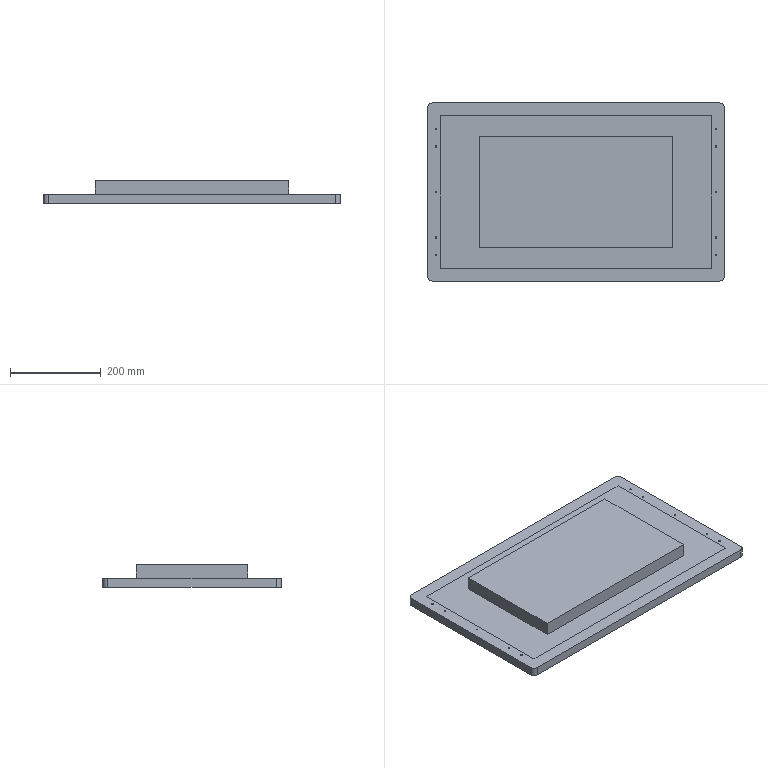Part | SolidWorks | features BaseBody 2 | 2 solids | 55 faces | box 654.7 x 392.6 x 50 mm | volume 8081843 mm3 | plane 31 | cylinder 24 | commonest cylinder face diameters 3.2 x20 20 x4
STEP:
#1=CARTESIAN_POINT('',(299.,168.,1.));
#2=VERTEX_POINT('',#1);
#3=CARTESIAN_POINT('',(299.,-168.,1.));
#4=VERTEX_POINT('',#3);
#5=CARTESIAN_POINT('',(299.,-168.,1.));
#6=DIRECTION('',(0.,-1.,0.));
#7=VECTOR('',#6,1000.);
#8=LINE('',#5,#7);
#9=EDGE_CURVE('',#2,#4,#8,.T.);
#10=ORIENTED_EDGE('',*,*,#9,.F.);
#11=CARTESIAN_POINT('',(299.,168.,20.));
#12=VERTEX_POINT('',#11);
#13=CARTESIAN_POINT('',(299.,168.,50.01));
#14=DIRECTION('',(0.,0.,-1.));
#15=VECTOR('',#14,1000.);
#16=LINE('',#13,#15);
#17=EDGE_CURVE('',#12,#2,#16,.T.);
#18=ORIENTED_EDGE('',*,*,#17,.F.);
#19=CARTESIAN_POINT('',(299.,-168.,20.));
#20=VERTEX_POINT('',#19);
#21=CARTESIAN_POINT('',(299.,0.,20.));
#22=DIRECTION('',(0.,-1.,0.));
#23=VECTOR('',#22,1000.);
#24=LINE('',#21,#23);
#25=EDGE_CURVE('',#12,#20,#24,.T.);
#26=ORIENTED_EDGE('',*,*,#25,.T.);
#27=CARTESIAN_POINT('',(299.,-168.,50.01));
#28=DIRECTION('',(0.,0.,-1.));
#29=VECTOR('',#28,1000.);
#30=LINE('',#27,#29);
#31=EDGE_CURVE('',#20,#4,#30,.T.);
#32=ORIENTED_EDGE('',*,*,#31,.T.);
#33=EDGE_LOOP('',(#10,#18,#26,#32));
#34=FACE_OUTER_BOUND('',#33,.T.);
#35=CARTESIAN_POINT('',(299.,168.,50.01));
#36=DIRECTION('',(1.,0.,0.));
#37=DIRECTION('',(0.,1.,0.));
#38=AXIS2_PLACEMENT_3D('',#35,#36,#37);
#39=PLANE('',#38);
#40=ADVANCED_FACE('',(#34),#39,.T.);
#41=CARTESIAN_POINT('',(-299.,168.,1.));
#42=VERTEX_POINT('',#41);
#43=CARTESIAN_POINT('',(299.,168.,1.));
#44=DIRECTION('',(1.,0.,0.));
#45=VECTOR('',#44,1000.);
#46=LINE('',#43,#45);
#47=EDGE_CURVE('',#42,#2,#46,.T.);
#48=ORIENTED_EDGE('',*,*,#47,.F.);
#49=CARTESIAN_POINT('',(-299.,168.,20.));
#50=VERTEX_POINT('',#49);
#51=CARTESIAN_POINT('',(-299.,168.,50.01));
#52=DIRECTION('',(0.,0.,-1.));
#53=VECTOR('',#52,1000.);
#54=LINE('',#51,#53);
#55=EDGE_CURVE('',#50,#42,#54,.T.);
#56=ORIENTED_EDGE('',*,*,#55,.F.);
#57=CARTESIAN_POINT('',(0.,168.,20.));
#58=DIRECTION('',(1.,0.,0.));
#59=VECTOR('',#58,1000.);
#60=LINE('',#57,#59);
#61=EDGE_CURVE('',#50,#12,#60,.T.);
#62=ORIENTED_EDGE('',*,*,#61,.T.);
#63=ORIENTED_EDGE('',*,*,#17,.T.);
#64=EDGE_LOOP('',(#48,#56,#62,#63));
#65=FACE_OUTER_BOUND('',#64,.T.);
#66=CARTESIAN_POINT('',(-299.,168.,50.01));
#67=DIRECTION('',(0.,1.,0.));
#68=DIRECTION('',(1.,0.,0.));
#69=AXIS2_PLACEMENT_3D('',#66,#67,#68);
#70=PLANE('',#69);
#71=ADVANCED_FACE('',(#65),#70,.T.);
#72=CARTESIAN_POINT('',(-299.,-168.,1.));
#73=VERTEX_POINT('',#72);
#74=CARTESIAN_POINT('',(-299.,-168.,1.));
#75=DIRECTION('',(0.,1.,0.));
#76=VECTOR('',#75,1000.);
#77=LINE('',#74,#76);
#78=EDGE_CURVE('',#73,#42,#77,.T.);
#79=ORIENTED_EDGE('',*,*,#78,.F.);
#80=CARTESIAN_POINT('',(-299.,-168.,20.));
#81=VERTEX_POINT('',#80);
#82=CARTESIAN_POINT('',(-299.,-168.,50.01));
#83=DIRECTION('',(0.,0.,-1.));
#84=VECTOR('',#83,1000.);
#85=LINE('',#82,#84);
#86=EDGE_CURVE('',#81,#73,#85,.T.);
#87=ORIENTED_EDGE('',*,*,#86,.F.);
#88=CARTESIAN_POINT('',(-299.,0.,20.));
#89=DIRECTION('',(0.,1.,0.));
#90=VECTOR('',#89,1000.);
#91=LINE('',#88,#90);
#92=EDGE_CURVE('',#81,#50,#91,.T.);
#93=ORIENTED_EDGE('',*,*,#92,.T.);
#94=ORIENTED_EDGE('',*,*,#55,.T.);
#95=EDGE_LOOP('',(#79,#87,#93,#94));
#96=FACE_OUTER_BOUND('',#95,.T.);
#97=CARTESIAN_POINT('',(-299.,-168.,50.01));
#98=DIRECTION('',(-1.,0.,0.));
#99=DIRECTION('',(0.,0.,1.));
#100=AXIS2_PLACEMENT_3D('',#97,#98,#99);
#101=PLANE('',#100);
#102=ADVANCED_FACE('',(#96),#101,.T.);
#103=CARTESIAN_POINT('',(299.,-168.,1.));
#104=DIRECTION('',(-1.,0.,0.));
#105=VECTOR('',#104,1000.);
#106=LINE('',#103,#105);
#107=EDGE_CURVE('',#4,#73,#106,.T.);
#108=ORIENTED_EDGE('',*,*,#107,.F.);
#109=ORIENTED_EDGE('',*,*,#31,.F.);
#110=CARTESIAN_POINT('',(0.,-168.,20.));
#111=DIRECTION('',(-1.,0.,0.));
#112=VECTOR('',#111,1000.);
#113=LINE('',#110,#112);
#114=EDGE_CURVE('',#20,#81,#113,.T.);
#115=ORIENTED_EDGE('',*,*,#114,.T.);
#116=ORIENTED_EDGE('',*,*,#86,.T.);
#117=EDGE_LOOP('',(#108,#109,#115,#116));
#118=FACE_OUTER_BOUND('',#117,.T.);
#119=CARTESIAN_POINT('',(299.,-168.,50.01));
#120=DIRECTION('',(0.,-1.,0.));
#121=DIRECTION('',(0.,0.,-1.));
#122=AXIS2_PLACEMENT_3D('',#119,#120,#121);
#123=PLANE('',#122);
#124=ADVANCED_FACE('',(#118),#123,.T.);
#125=ORIENTED_EDGE('',*,*,#78,.T.);
#126=ORIENTED_EDGE('',*,*,#47,.T.);
#127=ORIENTED_EDGE('',*,*,#9,.T.);
#128=ORIENTED_EDGE('',*,*,#107,.T.);
#129=EDGE_LOOP('',(#125,#126,#127,#128));
#130=FACE_OUTER_BOUND('',#129,.T.);
#131=CARTESIAN_POINT('',(0.,0.,1.));
#132=DIRECTION('',(0.,0.,1.));
#133=DIRECTION('',(1.,0.,0.));
#134=AXIS2_PLACEMENT_3D('',#131,#132,#133);
#135=PLANE('',#134);
#136=ADVANCED_FACE('',(#130),#135,.F.);
#137=CARTESIAN_POINT('',(213.,-123.,20.));
#138=VERTEX_POINT('',#137);
#139=CARTESIAN_POINT('',(213.,123.,20.));
#140=VERTEX_POINT('',#139);
#141=CARTESIAN_POINT('',(213.,-123.,20.));
#142=DIRECTION('',(0.,1.,0.));
#143=VECTOR('',#142,1000.);
#144=LINE('',#141,#143);
#145=EDGE_CURVE('',#138,#140,#144,.T.);
#146=ORIENTED_EDGE('',*,*,#145,.F.);
#147=CARTESIAN_POINT('',(-213.,-123.,20.));
#148=VERTEX_POINT('',#147);
#149=CARTESIAN_POINT('',(-213.,-123.,20.));
#150=DIRECTION('',(1.,0.,0.));
#151=VECTOR('',#150,1000.);
#152=LINE('',#149,#151);
#153=EDGE_CURVE('',#148,#138,#152,.T.);
#154=ORIENTED_EDGE('',*,*,#153,.F.);
#155=CARTESIAN_POINT('',(-213.,123.,20.));
#156=VERTEX_POINT('',#155);
#157=CARTESIAN_POINT('',(-213.,-123.,20.));
#158=DIRECTION('',(0.,-1.,0.));
#159=VECTOR('',#158,1000.);
#160=LINE('',#157,#159);
#161=EDGE_CURVE('',#156,#148,#160,.T.);
#162=ORIENTED_EDGE('',*,*,#161,.F.);
#163=CARTESIAN_POINT('',(-213.,123.,20.));
#164=DIRECTION('',(-1.,0.,0.));
#165=VECTOR('',#164,1000.);
#166=LINE('',#163,#165);
#167=EDGE_CURVE('',#140,#156,#166,.T.);
#168=ORIENTED_EDGE('',*,*,#167,.F.);
#169=EDGE_LOOP('',(#146,#154,#162,#168));
#170=FACE_BOUND('',#169,.T.);
#171=ORIENTED_EDGE('',*,*,#114,.F.);
#172=ORIENTED_EDGE('',*,*,#25,.F.);
#173=ORIENTED_EDGE('',*,*,#61,.F.);
#174=ORIENTED_EDGE('',*,*,#92,.F.);
#175=EDGE_LOOP('',(#171,#172,#173,#174));
#176=FACE_OUTER_BOUND('',#175,.T.);
#177=CARTESIAN_POINT('',(0.,0.,20.));
#178=DIRECTION('',(0.,0.,-1.));
#179=DIRECTION('',(0.,-1.,0.));
#180=AXIS2_PLACEMENT_3D('',#177,#178,#179);
#181=PLANE('',#180);
#182=ADVANCED_FACE('',(#170,#176),#181,.F.);
#183=ORIENTED_EDGE('',*,*,#145,.T.);
#184=CARTESIAN_POINT('',(213.,123.,50.));
#185=VERTEX_POINT('',#184);
#186=CARTESIAN_POINT('',(213.,123.,50.));
#187=DIRECTION('',(0.,0.,-1.));
#188=VECTOR('',#187,1000.);
#189=LINE('',#186,#188);
#190=EDGE_CURVE('',#185,#140,#189,.T.);
#191=ORIENTED_EDGE('',*,*,#190,.F.);
#192=CARTESIAN_POINT('',(213.,-123.,50.));
#193=VERTEX_POINT('',#192);
#194=CARTESIAN_POINT('',(213.,-123.,50.));
#195=DIRECTION('',(0.,1.,0.));
#196=VECTOR('',#195,1000.);
#197=LINE('',#194,#196);
#198=EDGE_CURVE('',#193,#185,#197,.T.);
#199=ORIENTED_EDGE('',*,*,#198,.F.);
#200=CARTESIAN_POINT('',(213.,-123.,50.));
#201=DIRECTION('',(0.,0.,-1.));
#202=VECTOR('',#201,1000.);
#203=LINE('',#200,#202);
#204=EDGE_CURVE('',#193,#138,#203,.T.);
#205=ORIENTED_EDGE('',*,*,#204,.T.);
#206=EDGE_LOOP('',(#183,#191,#199,#205));
#207=FACE_OUTER_BOUND('',#206,.T.);
#208=CARTESIAN_POINT('',(213.,-123.,50.));
#209=DIRECTION('',(-1.,0.,0.));
#210=DIRECTION('',(0.,0.,1.));
#211=AXIS2_PLACEMENT_3D('',#208,#209,#210);
#212=PLANE('',#211);
#213=ADVANCED_FACE('',(#207),#212,.F.);
#214=ORIENTED_EDGE('',*,*,#153,.T.);
#215=ORIENTED_EDGE('',*,*,#204,.F.);
#216=CARTESIAN_POINT('',(-213.,-123.,50.));
#217=VERTEX_POINT('',#216);
#218=CARTESIAN_POINT('',(-213.,-123.,50.));
#219=DIRECTION('',(1.,0.,0.));
#220=VECTOR('',#219,1000.);
#221=LINE('',#218,#220);
#222=EDGE_CURVE('',#217,#193,#221,.T.);
#223=ORIENTED_EDGE('',*,*,#222,.F.);
#224=CARTESIAN_POINT('',(-213.,-123.,50.));
#225=DIRECTION('',(0.,0.,-1.));
#226=VECTOR('',#225,1000.);
#227=LINE('',#224,#226);
#228=EDGE_CURVE('',#217,#148,#227,.T.);
#229=ORIENTED_EDGE('',*,*,#228,.T.);
#230=EDGE_LOOP('',(#214,#215,#223,#229));
#231=FACE_OUTER_BOUND('',#230,.T.);
#232=CARTESIAN_POINT('',(-213.,-123.,50.));
#233=DIRECTION('',(0.,1.,0.));
#234=DIRECTION('',(1.,0.,0.));
#235=AXIS2_PLACEMENT_3D('',#232,#233,#234);
#236=PLANE('',#235);
#237=ADVANCED_FACE('',(#231),#236,.F.);
#238=ORIENTED_EDGE('',*,*,#161,.T.);
#239=ORIENTED_EDGE('',*,*,#228,.F.);
#240=CARTESIAN_POINT('',(-213.,123.,50.));
#241=VERTEX_POINT('',#240);
#242=CARTESIAN_POINT('',(-213.,-123.,50.));
#243=DIRECTION('',(0.,-1.,0.));
#244=VECTOR('',#243,1000.);
#245=LINE('',#242,#244);
#246=EDGE_CURVE('',#241,#217,#245,.T.);
#247=ORIENTED_EDGE('',*,*,#246,.F.);
#248=CARTESIAN_POINT('',(-213.,123.,50.));
#249=DIRECTION('',(0.,0.,-1.));
#250=VECTOR('',#249,1000.);
#251=LINE('',#248,#250);
#252=EDGE_CURVE('',#241,#156,#251,.T.);
#253=ORIENTED_EDGE('',*,*,#252,.T.);
#254=EDGE_LOOP('',(#238,#239,#247,#253));
#255=FACE_OUTER_BOUND('',#254,.T.);
#256=CARTESIAN_POINT('',(-213.,-123.,50.));
#257=DIRECTION('',(1.,0.,0.));
#258=DIRECTION('',(0.,1.,0.));
#259=AXIS2_PLACEMENT_3D('',#256,#257,#258);
#260=PLANE('',#259);
#261=ADVANCED_FACE('',(#255),#260,.F.);
#262=ORIENTED_EDGE('',*,*,#167,.T.);
#263=ORIENTED_EDGE('',*,*,#252,.F.);
#264=CARTESIAN_POINT('',(-213.,123.,50.));
#265=DIRECTION('',(-1.,0.,0.));
#266=VECTOR('',#265,1000.);
#267=LINE('',#264,#266);
#268=EDGE_CURVE('',#185,#241,#267,.T.);
#269=ORIENTED_EDGE('',*,*,#268,.F.);
#270=ORIENTED_EDGE('',*,*,#190,.T.);
#271=EDGE_LOOP('',(#262,#263,#269,#270));
#272=FACE_OUTER_BOUND('',#271,.T.);
#273=CARTESIAN_POINT('',(-213.,123.,50.));
#274=DIRECTION('',(0.,-1.,0.));
#275=DIRECTION('',(0.,0.,-1.));
#276=AXIS2_PLACEMENT_3D('',#273,#274,#275);
#277=PLANE('',#276);
#278=ADVANCED_FACE('',(#272),#277,.F.);
#279=ORIENTED_EDGE('',*,*,#198,.T.);
#280=ORIENTED_EDGE('',*,*,#268,.T.);
#281=ORIENTED_EDGE('',*,*,#246,.T.);
#282=ORIENTED_EDGE('',*,*,#222,.T.);
#283=EDGE_LOOP('',(#279,#280,#281,#282));
#284=FACE_OUTER_BOUND('',#283,.T.);
#285=CARTESIAN_POINT('',(0.,0.,50.));
#286=DIRECTION('',(0.,0.,-1.));
#287=DIRECTION('',(0.,-1.,0.));
#288=AXIS2_PLACEMENT_3D('',#285,#286,#287);
#289=PLANE('',#288);
#290=ADVANCED_FACE('',(#284),#289,.F.);
#291=CLOSED_SHELL('',(#40,#71,#102,#124,#136,#182,#213,#237,#261,#278,#290));
#292=MANIFOLD_SOLID_BREP('',#291);
#293=CARTESIAN_POINT('',(317.35,-196.3,20.));
#294=VERTEX_POINT('',#293);
#295=CARTESIAN_POINT('',(327.35,-186.3,20.));
#296=VERTEX_POINT('',#295);
#297=CARTESIAN_POINT('',(317.35,-186.3,20.));
#298=DIRECTION('',(0.,0.,1.));
#299=DIRECTION('',(-1.,0.,0.));
#300=AXIS2_PLACEMENT_3D('',#297,#298,#299);
#301=CIRCLE('',#300,10.);
#302=EDGE_CURVE('',#294,#296,#301,.T.);
#303=ORIENTED_EDGE('',*,*,#302,.F.);
#304=CARTESIAN_POINT('',(317.35,-196.3,0.));
#305=VERTEX_POINT('',#304);
#306=CARTESIAN_POINT('',(317.35,-196.3,20.));
#307=DIRECTION('',(0.,0.,1.));
#308=VECTOR('',#307,1000.);
#309=LINE('',#306,#308);
#310=EDGE_CURVE('',#305,#294,#309,.T.);
#311=ORIENTED_EDGE('',*,*,#310,.F.);
#312=CARTESIAN_POINT('',(327.35,-186.3,0.));
#313=VERTEX_POINT('',#312);
#314=CARTESIAN_POINT('',(317.35,-186.3,0.));
#315=DIRECTION('',(0.,0.,-1.));
#316=DIRECTION('',(-1.,0.,0.));
#317=AXIS2_PLACEMENT_3D('',#314,#315,#316);
#318=CIRCLE('',#317,10.);
#319=EDGE_CURVE('',#313,#305,#318,.T.);
#320=ORIENTED_EDGE('',*,*,#319,.F.);
#321=CARTESIAN_POINT('',(327.35,-186.3,20.));
#322=DIRECTION('',(0.,0.,-1.));
#323=VECTOR('',#322,1000.);
#324=LINE('',#321,#323);
#325=EDGE_CURVE('',#296,#313,#324,.T.);
#326=ORIENTED_EDGE('',*,*,#325,.F.);
#327=EDGE_LOOP('',(#303,#311,#320,#326));
#328=FACE_OUTER_BOUND('',#327,.T.);
#329=CARTESIAN_POINT('',(317.35,-186.3,20.));
#330=DIRECTION('',(0.,0.,-1.));
#331=DIRECTION('',(-1.,0.,0.));
#332=AXIS2_PLACEMENT_3D('',#329,#330,#331);
#333=CYLINDRICAL_SURFACE('',#332,10.);
#334=ADVANCED_FACE('',(#328),#333,.T.);
#335=CARTESIAN_POINT('',(327.35,186.3,20.));
#336=VERTEX_POINT('',#335);
#337=CARTESIAN_POINT('',(317.35,196.3,20.));
#338=VERTEX_POINT('',#337);
#339=CARTESIAN_POINT('',(317.35,186.3,20.));
#340=DIRECTION('',(0.,0.,1.));
#341=DIRECTION('',(-1.,0.,0.));
#342=AXIS2_PLACEMENT_3D('',#339,#340,#341);
#343=CIRCLE('',#342,10.);
#344=EDGE_CURVE('',#336,#338,#343,.T.);
#345=ORIENTED_EDGE('',*,*,#344,.F.);
#346=CARTESIAN_POINT('',(327.35,186.3,0.));
#347=VERTEX_POINT('',#346);
#348=CARTESIAN_POINT('',(327.35,186.3,20.));
#349=DIRECTION('',(0.,0.,1.));
#350=VECTOR('',#349,1000.);
#351=LINE('',#348,#350);
#352=EDGE_CURVE('',#347,#336,#351,.T.);
#353=ORIENTED_EDGE('',*,*,#352,.F.);
#354=CARTESIAN_POINT('',(317.35,196.3,0.));
#355=VERTEX_POINT('',#354);
#356=CARTESIAN_POINT('',(317.35,186.3,0.));
#357=DIRECTION('',(0.,0.,-1.));
#358=DIRECTION('',(-1.,0.,0.));
#359=AXIS2_PLACEMENT_3D('',#356,#357,#358);
#360=CIRCLE('',#359,10.);
#361=EDGE_CURVE('',#355,#347,#360,.T.);
#362=ORIENTED_EDGE('',*,*,#361,.F.);
#363=CARTESIAN_POINT('',(317.35,196.3,20.));
#364=DIRECTION('',(0.,0.,-1.));
#365=VECTOR('',#364,1000.);
#366=LINE('',#363,#365);
#367=EDGE_CURVE('',#338,#355,#366,.T.);
#368=ORIENTED_EDGE('',*,*,#367,.F.);
#369=EDGE_LOOP('',(#345,#353,#362,#368));
#370=FACE_OUTER_BOUND('',#369,.T.);
#371=CARTESIAN_POINT('',(317.35,186.3,20.));
#372=DIRECTION('',(0.,0.,-1.));
#373=DIRECTION('',(-1.,0.,0.));
#374=AXIS2_PLACEMENT_3D('',#371,#372,#373);
#375=CYLINDRICAL_SURFACE('',#374,10.);
#376=ADVANCED_FACE('',(#370),#375,.T.);
#377=CARTESIAN_POINT('',(-317.35,196.3,20.));
#378=VERTEX_POINT('',#377);
#379=CARTESIAN_POINT('',(-327.35,186.3,20.));
#380=VERTEX_POINT('',#379);
#381=CARTESIAN_POINT('',(-317.35,186.3,20.));
#382=DIRECTION('',(0.,0.,1.));
#383=DIRECTION('',(-1.,0.,0.));
#384=AXIS2_PLACEMENT_3D('',#381,#382,#383);
#385=CIRCLE('',#384,10.);
#386=EDGE_CURVE('',#378,#380,#385,.T.);
#387=ORIENTED_EDGE('',*,*,#386,.F.);
#388=CARTESIAN_POINT('',(-317.35,196.3,0.));
#389=VERTEX_POINT('',#388);
#390=CARTESIAN_POINT('',(-317.35,196.3,20.));
#391=DIRECTION('',(0.,0.,1.));
#392=VECTOR('',#391,1000.);
#393=LINE('',#390,#392);
#394=EDGE_CURVE('',#389,#378,#393,.T.);
#395=ORIENTED_EDGE('',*,*,#394,.F.);
#396=CARTESIAN_POINT('',(-327.35,186.3,0.));
#397=VERTEX_POINT('',#396);
#398=CARTESIAN_POINT('',(-317.35,186.3,0.));
#399=DIRECTION('',(0.,0.,-1.));
#400=DIRECTION('',(-1.,0.,0.));
#401=AXIS2_PLACEMENT_3D('',#398,#399,#400);
#402=CIRCLE('',#401,10.);
#403=EDGE_CURVE('',#397,#389,#402,.T.);
#404=ORIENTED_EDGE('',*,*,#403,.F.);
#405=CARTESIAN_POINT('',(-327.35,186.3,20.));
#406=DIRECTION('',(0.,0.,-1.));
#407=VECTOR('',#406,1000.);
#408=LINE('',#405,#407);
#409=EDGE_CURVE('',#380,#397,#408,.T.);
#410=ORIENTED_EDGE('',*,*,#409,.F.);
#411=EDGE_LOOP('',(#387,#395,#404,#410));
#412=FACE_OUTER_BOUND('',#411,.T.);
#413=CARTESIAN_POINT('',(-317.35,186.3,20.));
#414=DIRECTION('',(0.,0.,-1.));
#415=DIRECTION('',(-1.,0.,0.));
#416=AXIS2_PLACEMENT_3D('',#413,#414,#415);
#417=CYLINDRICAL_SURFACE('',#416,10.);
#418=ADVANCED_FACE('',(#412),#417,.T.);
#419=CARTESIAN_POINT('',(-327.35,-186.3,20.));
#420=VERTEX_POINT('',#419);
#421=CARTESIAN_POINT('',(-317.35,-196.3,20.));
#422=VERTEX_POINT('',#421);
#423=CARTESIAN_POINT('',(-317.35,-186.3,20.));
#424=DIRECTION('',(0.,0.,1.));
#425=DIRECTION('',(-1.,0.,0.));
#426=AXIS2_PLACEMENT_3D('',#423,#424,#425);
#427=CIRCLE('',#426,10.);
#428=EDGE_CURVE('',#420,#422,#427,.T.);
#429=ORIENTED_EDGE('',*,*,#428,.F.);
#430=CARTESIAN_POINT('',(-327.35,-186.3,0.));
#431=VERTEX_POINT('',#430);
#432=CARTESIAN_POINT('',(-327.35,-186.3,20.));
#433=DIRECTION('',(0.,0.,1.));
#434=VECTOR('',#433,1000.);
#435=LINE('',#432,#434);
#436=EDGE_CURVE('',#431,#420,#435,.T.);
#437=ORIENTED_EDGE('',*,*,#436,.F.);
#438=CARTESIAN_POINT('',(-317.35,-196.3,0.));
#439=VERTEX_POINT('',#438);
#440=CARTESIAN_POINT('',(-317.35,-186.3,0.));
#441=DIRECTION('',(0.,0.,-1.));
#442=DIRECTION('',(-1.,0.,0.));
#443=AXIS2_PLACEMENT_3D('',#440,#441,#442);
#444=CIRCLE('',#443,10.);
#445=EDGE_CURVE('',#439,#431,#444,.T.);
#446=ORIENTED_EDGE('',*,*,#445,.F.);
#447=CARTESIAN_POINT('',(-317.35,-196.3,20.));
#448=DIRECTION('',(0.,0.,-1.));
#449=VECTOR('',#448,1000.);
#450=LINE('',#447,#449);
#451=EDGE_CURVE('',#422,#439,#450,.T.);
#452=ORIENTED_EDGE('',*,*,#451,.F.);
#453=EDGE_LOOP('',(#429,#437,#446,#452));
#454=FACE_OUTER_BOUND('',#453,.T.);
#455=CARTESIAN_POINT('',(-317.35,-186.3,20.));
#456=DIRECTION('',(0.,0.,-1.));
#457=DIRECTION('',(-1.,0.,0.));
#458=AXIS2_PLACEMENT_3D('',#455,#456,#457);
#459=CYLINDRICAL_SURFACE('',#458,10.);
#460=ADVANCED_FACE('',(#454),#459,.T.);
#461=CARTESIAN_POINT('',(-307.45,138.8,18.8));
#462=VERTEX_POINT('',#461);
#463=CARTESIAN_POINT('',(-310.65,138.8,18.8));
#464=VERTEX_POINT('',#463);
#465=CARTESIAN_POINT('',(-309.05,138.8,18.8));
#466=DIRECTION('',(0.,0.,1.));
#467=DIRECTION('',(-1.,0.,0.));
#468=AXIS2_PLACEMENT_3D('',#465,#466,#467);
#469=CIRCLE('',#468,1.6);
#470=EDGE_CURVE('',#462,#464,#469,.T.);
#471=ORIENTED_EDGE('',*,*,#470,.T.);
#472=CARTESIAN_POINT('',(-309.05,138.8,18.8));
#473=DIRECTION('',(0.,0.,1.));
#474=DIRECTION('',(-1.,0.,0.));
#475=AXIS2_PLACEMENT_3D('',#472,#473,#474);
#476=CIRCLE('',#475,1.6);
#477=EDGE_CURVE('',#464,#462,#476,.T.);
#478=ORIENTED_EDGE('',*,*,#477,.T.);
#479=EDGE_LOOP('',(#471,#478));
#480=FACE_OUTER_BOUND('',#479,.T.);
#481=CARTESIAN_POINT('',(-309.05,138.8,18.8));
#482=DIRECTION('',(0.,0.,-1.));
#483=DIRECTION('',(0.,-1.,0.));
#484=AXIS2_PLACEMENT_3D('',#481,#482,#483);
#485=PLANE('',#484);
#486=ADVANCED_FACE('',(#480),#485,.F.);
#487=CARTESIAN_POINT('',(-307.45,100.,18.8));
#488=VERTEX_POINT('',#487);
#489=CARTESIAN_POINT('',(-310.65,100.,18.8));
#490=VERTEX_POINT('',#489);
#491=CARTESIAN_POINT('',(-309.05,100.,18.8));
#492=DIRECTION('',(0.,0.,1.));
#493=DIRECTION('',(-1.,0.,0.));
#494=AXIS2_PLACEMENT_3D('',#491,#492,#493);
#495=CIRCLE('',#494,1.6);
#496=EDGE_CURVE('',#488,#490,#495,.T.);
#497=ORIENTED_EDGE('',*,*,#496,.T.);
#498=CARTESIAN_POINT('',(-309.05,100.,18.8));
#499=DIRECTION('',(0.,0.,1.));
#500=DIRECTION('',(-1.,0.,0.));
#501=AXIS2_PLACEMENT_3D('',#498,#499,#500);
#502=CIRCLE('',#501,1.6);
#503=EDGE_CURVE('',#490,#488,#502,.T.);
#504=ORIENTED_EDGE('',*,*,#503,.T.);
#505=EDGE_LOOP('',(#497,#504));
#506=FACE_OUTER_BOUND('',#505,.T.);
#507=CARTESIAN_POINT('',(-309.05,100.,18.8));
#508=DIRECTION('',(0.,0.,-1.));
#509=DIRECTION('',(0.,-1.,0.));
#510=AXIS2_PLACEMENT_3D('',#507,#508,#509);
#511=PLANE('',#510);
#512=ADVANCED_FACE('',(#506),#511,.F.);
#513=CARTESIAN_POINT('',(-307.45,0.,18.8));
#514=VERTEX_POINT('',#513);
#515=CARTESIAN_POINT('',(-310.65,0.,18.8));
#516=VERTEX_POINT('',#515);
#517=CARTESIAN_POINT('',(-309.05,0.,18.8));
#518=DIRECTION('',(0.,0.,1.));
#519=DIRECTION('',(-1.,0.,0.));
#520=AXIS2_PLACEMENT_3D('',#517,#518,#519);
#521=CIRCLE('',#520,1.6);
#522=EDGE_CURVE('',#514,#516,#521,.T.);
#523=ORIENTED_EDGE('',*,*,#522,.T.);
#524=CARTESIAN_POINT('',(-309.05,0.,18.8));
#525=DIRECTION('',(0.,0.,1.));
#526=DIRECTION('',(-1.,0.,0.));
#527=AXIS2_PLACEMENT_3D('',#524,#525,#526);
#528=CIRCLE('',#527,1.6);
#529=EDGE_CURVE('',#516,#514,#528,.T.);
#530=ORIENTED_EDGE('',*,*,#529,.T.);
#531=EDGE_LOOP('',(#523,#530));
#532=FACE_OUTER_BOUND('',#531,.T.);
#533=CARTESIAN_POINT('',(-309.05,0.,18.8));
#534=DIRECTION('',(0.,0.,-1.));
#535=DIRECTION('',(0.,-1.,0.));
#536=AXIS2_PLACEMENT_3D('',#533,#534,#535);
#537=PLANE('',#536);
#538=ADVANCED_FACE('',(#532),#537,.F.);
#539=CARTESIAN_POINT('',(-307.45,-100.,18.8));
#540=VERTEX_POINT('',#539);
#541=CARTESIAN_POINT('',(-310.65,-100.,18.8));
#542=VERTEX_POINT('',#541);
#543=CARTESIAN_POINT('',(-309.05,-100.,18.8));
#544=DIRECTION('',(0.,0.,1.));
#545=DIRECTION('',(1.,0.,0.));
#546=AXIS2_PLACEMENT_3D('',#543,#544,#545);
#547=CIRCLE('',#546,1.6);
#548=EDGE_CURVE('',#540,#542,#547,.T.);
#549=ORIENTED_EDGE('',*,*,#548,.T.);
#550=CARTESIAN_POINT('',(-309.05,-100.,18.8));
#551=DIRECTION('',(0.,0.,1.));
#552=DIRECTION('',(1.,0.,0.));
#553=AXIS2_PLACEMENT_3D('',#550,#551,#552);
#554=CIRCLE('',#553,1.6);
#555=EDGE_CURVE('',#542,#540,#554,.T.);
#556=ORIENTED_EDGE('',*,*,#555,.T.);
#557=EDGE_LOOP('',(#549,#556));
#558=FACE_OUTER_BOUND('',#557,.T.);
#559=CARTESIAN_POINT('',(-309.05,-100.,18.8));
#560=DIRECTION('',(0.,0.,1.));
#561=DIRECTION('',(1.,0.,0.));
#562=AXIS2_PLACEMENT_3D('',#559,#560,#561);
#563=PLANE('',#562);
#564=ADVANCED_FACE('',(#558),#563,.T.);
#565=CARTESIAN_POINT('',(-307.45,-138.8,18.8));
#566=VERTEX_POINT('',#565);
#567=CARTESIAN_POINT('',(-310.65,-138.8,18.8));
#568=VERTEX_POINT('',#567);
#569=CARTESIAN_POINT('',(-309.05,-138.8,18.8));
#570=DIRECTION('',(0.,0.,1.));
#571=DIRECTION('',(1.,0.,0.));
#572=AXIS2_PLACEMENT_3D('',#569,#570,#571);
#573=CIRCLE('',#572,1.6);
#574=EDGE_CURVE('',#566,#568,#573,.T.);
#575=ORIENTED_EDGE('',*,*,#574,.T.);
#576=CARTESIAN_POINT('',(-309.05,-138.8,18.8));
#577=DIRECTION('',(0.,0.,1.));
#578=DIRECTION('',(1.,0.,0.));
#579=AXIS2_PLACEMENT_3D('',#576,#577,#578);
#580=CIRCLE('',#579,1.6);
#581=EDGE_CURVE('',#568,#566,#580,.T.);
#582=ORIENTED_EDGE('',*,*,#581,.T.);
#583=EDGE_LOOP('',(#575,#582));
#584=FACE_OUTER_BOUND('',#583,.T.);
#585=CARTESIAN_POINT('',(-309.05,-138.8,18.8));
#586=DIRECTION('',(0.,0.,1.));
#587=DIRECTION('',(1.,0.,0.));
#588=AXIS2_PLACEMENT_3D('',#585,#586,#587);
#589=PLANE('',#588);
#590=ADVANCED_FACE('',(#584),#589,.T.);
#591=CARTESIAN_POINT('',(310.65,-138.8,18.8));
#592=VERTEX_POINT('',#591);
#593=CARTESIAN_POINT('',(307.45,-138.8,18.8));
#594=VERTEX_POINT('',#593);
#595=CARTESIAN_POINT('',(309.05,-138.8,18.8));
#596=DIRECTION('',(0.,0.,1.));
#597=DIRECTION('',(-1.,0.,0.));
#598=AXIS2_PLACEMENT_3D('',#595,#596,#597);
#599=CIRCLE('',#598,1.6);
#600=EDGE_CURVE('',#592,#594,#599,.T.);
#601=ORIENTED_EDGE('',*,*,#600,.T.);
#602=CARTESIAN_POINT('',(309.05,-138.8,18.8));
#603=DIRECTION('',(0.,0.,1.));
#604=DIRECTION('',(-1.,0.,0.));
#605=AXIS2_PLACEMENT_3D('',#602,#603,#604);
#606=CIRCLE('',#605,1.6);
#607=EDGE_CURVE('',#594,#592,#606,.T.);
#608=ORIENTED_EDGE('',*,*,#607,.T.);
#609=EDGE_LOOP('',(#601,#608));
#610=FACE_OUTER_BOUND('',#609,.T.);
#611=CARTESIAN_POINT('',(309.05,-138.8,18.8));
#612=DIRECTION('',(0.,0.,-1.));
#613=DIRECTION('',(0.,-1.,0.));
#614=AXIS2_PLACEMENT_3D('',#611,#612,#613);
#615=PLANE('',#614);
#616=ADVANCED_FACE('',(#610),#615,.F.);
#617=CARTESIAN_POINT('',(310.65,-100.,18.8));
#618=VERTEX_POINT('',#617);
#619=CARTESIAN_POINT('',(307.45,-100.,18.8));
#620=VERTEX_POINT('',#619);
#621=CARTESIAN_POINT('',(309.05,-100.,18.8));
#622=DIRECTION('',(0.,0.,1.));
#623=DIRECTION('',(-1.,0.,0.));
#624=AXIS2_PLACEMENT_3D('',#621,#622,#623);
#625=CIRCLE('',#624,1.6);
#626=EDGE_CURVE('',#618,#620,#625,.T.);
#627=ORIENTED_EDGE('',*,*,#626,.T.);
#628=CARTESIAN_POINT('',(309.05,-100.,18.8));
#629=DIRECTION('',(0.,0.,1.));
#630=DIRECTION('',(-1.,0.,0.));
#631=AXIS2_PLACEMENT_3D('',#628,#629,#630);
#632=CIRCLE('',#631,1.6);
#633=EDGE_CURVE('',#620,#618,#632,.T.);
#634=ORIENTED_EDGE('',*,*,#633,.T.);
#635=EDGE_LOOP('',(#627,#634));
#636=FACE_OUTER_BOUND('',#635,.T.);
#637=CARTESIAN_POINT('',(309.05,-100.,18.8));
#638=DIRECTION('',(0.,0.,-1.));
#639=DIRECTION('',(0.,-1.,0.));
#640=AXIS2_PLACEMENT_3D('',#637,#638,#639);
#641=PLANE('',#640);
#642=ADVANCED_FACE('',(#636),#641,.F.);
#643=CARTESIAN_POINT('',(310.65,0.,18.8));
#644=VERTEX_POINT('',#643);
#645=CARTESIAN_POINT('',(307.45,0.,18.8));
#646=VERTEX_POINT('',#645);
#647=CARTESIAN_POINT('',(309.05,0.,18.8));
#648=DIRECTION('',(0.,0.,1.));
#649=DIRECTION('',(1.,0.,0.));
#650=AXIS2_PLACEMENT_3D('',#647,#648,#649);
#651=CIRCLE('',#650,1.6);
#652=EDGE_CURVE('',#644,#646,#651,.T.);
#653=ORIENTED_EDGE('',*,*,#652,.T.);
#654=CARTESIAN_POINT('',(309.05,0.,18.8));
#655=DIRECTION('',(0.,0.,1.));
#656=DIRECTION('',(1.,0.,0.));
#657=AXIS2_PLACEMENT_3D('',#654,#655,#656);
#658=CIRCLE('',#657,1.6);
#659=EDGE_CURVE('',#646,#644,#658,.T.);
#660=ORIENTED_EDGE('',*,*,#659,.T.);
#661=EDGE_LOOP('',(#653,#660));
#662=FACE_OUTER_BOUND('',#661,.T.);
#663=CARTESIAN_POINT('',(309.05,0.,18.8));
#664=DIRECTION('',(0.,0.,1.));
#665=DIRECTION('',(1.,0.,0.));
#666=AXIS2_PLACEMENT_3D('',#663,#664,#665);
#667=PLANE('',#666);
#668=ADVANCED_FACE('',(#662),#667,.T.);
#669=CARTESIAN_POINT('',(310.65,100.,18.8));
#670=VERTEX_POINT('',#669);
#671=CARTESIAN_POINT('',(307.45,100.,18.8));
#672=VERTEX_POINT('',#671);
#673=CARTESIAN_POINT('',(309.05,100.,18.8));
#674=DIRECTION('',(0.,0.,1.));
#675=DIRECTION('',(1.,0.,0.));
#676=AXIS2_PLACEMENT_3D('',#673,#674,#675);
#677=CIRCLE('',#676,1.6);
#678=EDGE_CURVE('',#670,#672,#677,.T.);
#679=ORIENTED_EDGE('',*,*,#678,.T.);
#680=CARTESIAN_POINT('',(309.05,100.,18.8));
#681=DIRECTION('',(0.,0.,1.));
#682=DIRECTION('',(1.,0.,0.));
#683=AXIS2_PLACEMENT_3D('',#680,#681,#682);
#684=CIRCLE('',#683,1.6);
#685=EDGE_CURVE('',#672,#670,#684,.T.);
#686=ORIENTED_EDGE('',*,*,#685,.T.);
#687=EDGE_LOOP('',(#679,#686));
#688=FACE_OUTER_BOUND('',#687,.T.);
#689=CARTESIAN_POINT('',(309.05,100.,18.8));
#690=DIRECTION('',(0.,0.,1.));
#691=DIRECTION('',(1.,0.,0.));
#692=AXIS2_PLACEMENT_3D('',#689,#690,#691);
#693=PLANE('',#692);
#694=ADVANCED_FACE('',(#688),#693,.T.);
#695=CARTESIAN_POINT('',(310.65,138.8,18.8));
#696=VERTEX_POINT('',#695);
#697=CARTESIAN_POINT('',(307.45,138.8,18.8));
#698=VERTEX_POINT('',#697);
#699=CARTESIAN_POINT('',(309.05,138.8,18.8));
#700=DIRECTION('',(0.,0.,1.));
#701=DIRECTION('',(1.,0.,0.));
#702=AXIS2_PLACEMENT_3D('',#699,#700,#701);
#703=CIRCLE('',#702,1.6);
#704=EDGE_CURVE('',#696,#698,#703,.T.);
#705=ORIENTED_EDGE('',*,*,#704,.T.);
#706=CARTESIAN_POINT('',(309.05,138.8,18.8));
#707=DIRECTION('',(0.,0.,1.));
#708=DIRECTION('',(1.,0.,0.));
#709=AXIS2_PLACEMENT_3D('',#706,#707,#708);
#710=CIRCLE('',#709,1.6);
#711=EDGE_CURVE('',#698,#696,#710,.T.);
#712=ORIENTED_EDGE('',*,*,#711,.T.);
#713=EDGE_LOOP('',(#705,#712));
#714=FACE_OUTER_BOUND('',#713,.T.);
#715=CARTESIAN_POINT('',(309.05,138.8,18.8));
#716=DIRECTION('',(0.,0.,1.));
#717=DIRECTION('',(1.,0.,0.));
#718=AXIS2_PLACEMENT_3D('',#715,#716,#717);
#719=PLANE('',#718);
#720=ADVANCED_FACE('',(#714),#719,.T.);
#721=CARTESIAN_POINT('',(-327.35,-196.3,20.));
#722=DIRECTION('',(1.,0.,0.));
#723=VECTOR('',#722,1000.);
#724=LINE('',#721,#723);
#725=EDGE_CURVE('',#422,#294,#724,.T.);
#726=ORIENTED_EDGE('',*,*,#725,.F.);
#727=ORIENTED_EDGE('',*,*,#451,.T.);
#728=CARTESIAN_POINT('',(-327.35,-196.3,0.));
#729=DIRECTION('',(1.,0.,0.));
#730=VECTOR('',#729,1000.);
#731=LINE('',#728,#730);
#732=EDGE_CURVE('',#439,#305,#731,.T.);
#733=ORIENTED_EDGE('',*,*,#732,.T.);
#734=ORIENTED_EDGE('',*,*,#310,.T.);
#735=EDGE_LOOP('',(#726,#727,#733,#734));
#736=FACE_OUTER_BOUND('',#735,.T.);
#737=CARTESIAN_POINT('',(-327.35,-196.3,20.));
#738=DIRECTION('',(0.,1.,0.));
#739=DIRECTION('',(1.,0.,0.));
#740=AXIS2_PLACEMENT_3D('',#737,#738,#739);
#741=PLANE('',#740);
#742=ADVANCED_FACE('',(#736),#741,.F.);
#743=CARTESIAN_POINT('',(-327.35,-196.3,0.));
#744=DIRECTION('',(0.,-1.,0.));
#745=VECTOR('',#744,1000.);
#746=LINE('',#743,#745);
#747=EDGE_CURVE('',#397,#431,#746,.T.);
#748=ORIENTED_EDGE('',*,*,#747,.T.);
#749=ORIENTED_EDGE('',*,*,#436,.T.);
#750=CARTESIAN_POINT('',(-327.35,-196.3,20.));
#751=DIRECTION('',(0.,-1.,0.));
#752=VECTOR('',#751,1000.);
#753=LINE('',#750,#752);
#754=EDGE_CURVE('',#380,#420,#753,.T.);
#755=ORIENTED_EDGE('',*,*,#754,.F.);
#756=ORIENTED_EDGE('',*,*,#409,.T.);
#757=EDGE_LOOP('',(#748,#749,#755,#756));
#758=FACE_OUTER_BOUND('',#757,.T.);
#759=CARTESIAN_POINT('',(-327.35,-196.3,20.));
#760=DIRECTION('',(1.,0.,0.));
#761=DIRECTION('',(0.,1.,0.));
#762=AXIS2_PLACEMENT_3D('',#759,#760,#761);
#763=PLANE('',#762);
#764=ADVANCED_FACE('',(#758),#763,.F.);
#765=CARTESIAN_POINT('',(-327.35,196.3,0.));
#766=DIRECTION('',(-1.,0.,0.));
#767=VECTOR('',#766,1000.);
#768=LINE('',#765,#767);
#769=EDGE_CURVE('',#355,#389,#768,.T.);
#770=ORIENTED_EDGE('',*,*,#769,.T.);
#771=ORIENTED_EDGE('',*,*,#394,.T.);
#772=CARTESIAN_POINT('',(-327.35,196.3,20.));
#773=DIRECTION('',(-1.,0.,0.));
#774=VECTOR('',#773,1000.);
#775=LINE('',#772,#774);
#776=EDGE_CURVE('',#338,#378,#775,.T.);
#777=ORIENTED_EDGE('',*,*,#776,.F.);
#778=ORIENTED_EDGE('',*,*,#367,.T.);
#779=EDGE_LOOP('',(#770,#771,#777,#778));
#780=FACE_OUTER_BOUND('',#779,.T.);
#781=CARTESIAN_POINT('',(-327.35,196.3,20.));
#782=DIRECTION('',(0.,-1.,0.));
#783=DIRECTION('',(0.,0.,-1.));
#784=AXIS2_PLACEMENT_3D('',#781,#782,#783);
#785=PLANE('',#784);
#786=ADVANCED_FACE('',(#780),#785,.F.);
#787=CARTESIAN_POINT('',(327.35,-196.3,0.));
#788=DIRECTION('',(0.,1.,0.));
#789=VECTOR('',#788,1000.);
#790=LINE('',#787,#789);
#791=EDGE_CURVE('',#313,#347,#790,.T.);
#792=ORIENTED_EDGE('',*,*,#791,.T.);
#793=ORIENTED_EDGE('',*,*,#352,.T.);
#794=CARTESIAN_POINT('',(327.35,-196.3,20.));
#795=DIRECTION('',(0.,1.,0.));
#796=VECTOR('',#795,1000.);
#797=LINE('',#794,#796);
#798=EDGE_CURVE('',#296,#336,#797,.T.);
#799=ORIENTED_EDGE('',*,*,#798,.F.);
#800=ORIENTED_EDGE('',*,*,#325,.T.);
#801=EDGE_LOOP('',(#792,#793,#799,#800));
#802=FACE_OUTER_BOUND('',#801,.T.);
#803=CARTESIAN_POINT('',(327.35,-196.3,20.));
#804=DIRECTION('',(-1.,0.,0.));
#805=DIRECTION('',(0.,0.,1.));
#806=AXIS2_PLACEMENT_3D('',#803,#804,#805);
#807=PLANE('',#806);
#808=ADVANCED_FACE('',(#802),#807,.F.);
#809=ORIENTED_EDGE('',*,*,#477,.F.);
#810=CARTESIAN_POINT('',(-310.65,138.8,20.));
#811=VERTEX_POINT('',#810);
#812=CARTESIAN_POINT('',(-310.65,138.8,18.8));
#813=DIRECTION('',(0.,0.,1.));
#814=VECTOR('',#813,1000.);
#815=LINE('',#812,#814);
#816=EDGE_CURVE('',#464,#811,#815,.T.);
#817=ORIENTED_EDGE('',*,*,#816,.T.);
#818=CARTESIAN_POINT('',(-307.45,138.8,20.));
#819=VERTEX_POINT('',#818);
#820=CARTESIAN_POINT('',(-309.05,138.8,20.));
#821=DIRECTION('',(0.,0.,1.));
#822=DIRECTION('',(-1.,0.,0.));
#823=AXIS2_PLACEMENT_3D('',#820,#821,#822);
#824=CIRCLE('',#823,1.6);
#825=EDGE_CURVE('',#811,#819,#824,.T.);
#826=ORIENTED_EDGE('',*,*,#825,.T.);
#827=CARTESIAN_POINT('',(-307.45,138.8,18.8));
#828=DIRECTION('',(0.,0.,1.));
#829=VECTOR('',#828,1000.);
#830=LINE('',#827,#829);
#831=EDGE_CURVE('',#462,#819,#830,.T.);
#832=ORIENTED_EDGE('',*,*,#831,.F.);
#833=EDGE_LOOP('',(#809,#817,#826,#832));
#834=FACE_OUTER_BOUND('',#833,.T.);
#835=CARTESIAN_POINT('',(-309.05,138.8,18.8));
#836=DIRECTION('',(0.,0.,1.));
#837=DIRECTION('',(1.,0.,0.));
#838=AXIS2_PLACEMENT_3D('',#835,#836,#837);
#839=CYLINDRICAL_SURFACE('',#838,1.6);
#840=ADVANCED_FACE('',(#834),#839,.F.);
#841=ORIENTED_EDGE('',*,*,#816,.F.);
#842=ORIENTED_EDGE('',*,*,#470,.F.);
#843=ORIENTED_EDGE('',*,*,#831,.T.);
#844=CARTESIAN_POINT('',(-309.05,138.8,20.));
#845=DIRECTION('',(0.,0.,1.));
#846=DIRECTION('',(-1.,0.,0.));
#847=AXIS2_PLACEMENT_3D('',#844,#845,#846);
#848=CIRCLE('',#847,1.6);
#849=EDGE_CURVE('',#819,#811,#848,.T.);
#850=ORIENTED_EDGE('',*,*,#849,.T.);
#851=EDGE_LOOP('',(#841,#842,#843,#850));
#852=FACE_OUTER_BOUND('',#851,.T.);
#853=CARTESIAN_POINT('',(-309.05,138.8,18.8));
#854=DIRECTION('',(0.,0.,1.));
#855=DIRECTION('',(1.,0.,0.));
#856=AXIS2_PLACEMENT_3D('',#853,#854,#855);
#857=CYLINDRICAL_SURFACE('',#856,1.6);
#858=ADVANCED_FACE('',(#852),#857,.F.);
#859=ORIENTED_EDGE('',*,*,#503,.F.);
#860=CARTESIAN_POINT('',(-310.65,100.,20.));
#861=VERTEX_POINT('',#860);
#862=CARTESIAN_POINT('',(-310.65,100.,18.8));
#863=DIRECTION('',(0.,0.,1.));
#864=VECTOR('',#863,1000.);
#865=LINE('',#862,#864);
#866=EDGE_CURVE('',#490,#861,#865,.T.);
#867=ORIENTED_EDGE('',*,*,#866,.T.);
#868=CARTESIAN_POINT('',(-307.45,100.,20.));
#869=VERTEX_POINT('',#868);
#870=CARTESIAN_POINT('',(-309.05,100.,20.));
#871=DIRECTION('',(0.,0.,1.));
#872=DIRECTION('',(-1.,0.,0.));
#873=AXIS2_PLACEMENT_3D('',#870,#871,#872);
#874=CIRCLE('',#873,1.6);
#875=EDGE_CURVE('',#861,#869,#874,.T.);
#876=ORIENTED_EDGE('',*,*,#875,.T.);
#877=CARTESIAN_POINT('',(-307.45,100.,18.8));
#878=DIRECTION('',(0.,0.,1.));
#879=VECTOR('',#878,1000.);
#880=LINE('',#877,#879);
#881=EDGE_CURVE('',#488,#869,#880,.T.);
#882=ORIENTED_EDGE('',*,*,#881,.F.);
#883=EDGE_LOOP('',(#859,#867,#876,#882));
#884=FACE_OUTER_BOUND('',#883,.T.);
#885=CARTESIAN_POINT('',(-309.05,100.,18.8));
#886=DIRECTION('',(0.,0.,1.));
#887=DIRECTION('',(1.,0.,0.));
#888=AXIS2_PLACEMENT_3D('',#885,#886,#887);
#889=CYLINDRICAL_SURFACE('',#888,1.6);
#890=ADVANCED_FACE('',(#884),#889,.F.);
#891=ORIENTED_EDGE('',*,*,#866,.F.);
#892=ORIENTED_EDGE('',*,*,#496,.F.);
#893=ORIENTED_EDGE('',*,*,#881,.T.);
#894=CARTESIAN_POINT('',(-309.05,100.,20.));
#895=DIRECTION('',(0.,0.,1.));
#896=DIRECTION('',(-1.,0.,0.));
#897=AXIS2_PLACEMENT_3D('',#894,#895,#896);
#898=CIRCLE('',#897,1.6);
#899=EDGE_CURVE('',#869,#861,#898,.T.);
#900=ORIENTED_EDGE('',*,*,#899,.T.);
#901=EDGE_LOOP('',(#891,#892,#893,#900));
#902=FACE_OUTER_BOUND('',#901,.T.);
#903=CARTESIAN_POINT('',(-309.05,100.,18.8));
#904=DIRECTION('',(0.,0.,1.));
#905=DIRECTION('',(1.,0.,0.));
#906=AXIS2_PLACEMENT_3D('',#903,#904,#905);
#907=CYLINDRICAL_SURFACE('',#906,1.6);
#908=ADVANCED_FACE('',(#902),#907,.F.);
#909=ORIENTED_EDGE('',*,*,#529,.F.);
#910=CARTESIAN_POINT('',(-310.65,0.,20.));
#911=VERTEX_POINT('',#910);
#912=CARTESIAN_POINT('',(-310.65,0.,18.8));
#913=DIRECTION('',(0.,0.,1.));
#914=VECTOR('',#913,1000.);
#915=LINE('',#912,#914);
#916=EDGE_CURVE('',#516,#911,#915,.T.);
#917=ORIENTED_EDGE('',*,*,#916,.T.);
#918=CARTESIAN_POINT('',(-307.45,0.,20.));
#919=VERTEX_POINT('',#918);
#920=CARTESIAN_POINT('',(-309.05,0.,20.));
#921=DIRECTION('',(0.,0.,1.));
#922=DIRECTION('',(-1.,0.,0.));
#923=AXIS2_PLACEMENT_3D('',#920,#921,#922);
#924=CIRCLE('',#923,1.6);
#925=EDGE_CURVE('',#911,#919,#924,.T.);
#926=ORIENTED_EDGE('',*,*,#925,.T.);
#927=CARTESIAN_POINT('',(-307.45,0.,18.8));
#928=DIRECTION('',(0.,0.,1.));
#929=VECTOR('',#928,1000.);
#930=LINE('',#927,#929);
#931=EDGE_CURVE('',#514,#919,#930,.T.);
#932=ORIENTED_EDGE('',*,*,#931,.F.);
#933=EDGE_LOOP('',(#909,#917,#926,#932));
#934=FACE_OUTER_BOUND('',#933,.T.);
#935=CARTESIAN_POINT('',(-309.05,0.,18.8));
#936=DIRECTION('',(0.,0.,1.));
#937=DIRECTION('',(1.,0.,0.));
#938=AXIS2_PLACEMENT_3D('',#935,#936,#937);
#939=CYLINDRICAL_SURFACE('',#938,1.6);
#940=ADVANCED_FACE('',(#934),#939,.F.);
#941=ORIENTED_EDGE('',*,*,#916,.F.);
#942=ORIENTED_EDGE('',*,*,#522,.F.);
#943=ORIENTED_EDGE('',*,*,#931,.T.);
#944=CARTESIAN_POINT('',(-309.05,0.,20.));
#945=DIRECTION('',(0.,0.,1.));
#946=DIRECTION('',(-1.,0.,0.));
#947=AXIS2_PLACEMENT_3D('',#944,#945,#946);
#948=CIRCLE('',#947,1.6);
#949=EDGE_CURVE('',#919,#911,#948,.T.);
#950=ORIENTED_EDGE('',*,*,#949,.T.);
#951=EDGE_LOOP('',(#941,#942,#943,#950));
#952=FACE_OUTER_BOUND('',#951,.T.);
#953=CARTESIAN_POINT('',(-309.05,0.,18.8));
#954=DIRECTION('',(0.,0.,1.));
#955=DIRECTION('',(1.,0.,0.));
#956=AXIS2_PLACEMENT_3D('',#953,#954,#955);
#957=CYLINDRICAL_SURFACE('',#956,1.6);
#958=ADVANCED_FACE('',(#952),#957,.F.);
#959=ORIENTED_EDGE('',*,*,#555,.F.);
#960=CARTESIAN_POINT('',(-310.65,-100.,20.));
#961=VERTEX_POINT('',#960);
#962=CARTESIAN_POINT('',(-310.65,-100.,18.8));
#963=DIRECTION('',(0.,0.,1.));
#964=VECTOR('',#963,1000.);
#965=LINE('',#962,#964);
#966=EDGE_CURVE('',#542,#961,#965,.T.);
#967=ORIENTED_EDGE('',*,*,#966,.T.);
#968=CARTESIAN_POINT('',(-307.45,-100.,20.));
#969=VERTEX_POINT('',#968);
#970=CARTESIAN_POINT('',(-309.05,-100.,20.));
#971=DIRECTION('',(0.,0.,1.));
#972=DIRECTION('',(1.,0.,0.));
#973=AXIS2_PLACEMENT_3D('',#970,#971,#972);
#974=CIRCLE('',#973,1.6);
#975=EDGE_CURVE('',#961,#969,#974,.T.);
#976=ORIENTED_EDGE('',*,*,#975,.T.);
#977=CARTESIAN_POINT('',(-307.45,-100.,18.8));
#978=DIRECTION('',(0.,0.,1.));
#979=VECTOR('',#978,1000.);
#980=LINE('',#977,#979);
#981=EDGE_CURVE('',#540,#969,#980,.T.);
#982=ORIENTED_EDGE('',*,*,#981,.F.);
#983=EDGE_LOOP('',(#959,#967,#976,#982));
#984=FACE_OUTER_BOUND('',#983,.T.);
#985=CARTESIAN_POINT('',(-309.05,-100.,18.8));
#986=DIRECTION('',(0.,0.,1.));
#987=DIRECTION('',(1.,0.,0.));
#988=AXIS2_PLACEMENT_3D('',#985,#986,#987);
#989=CYLINDRICAL_SURFACE('',#988,1.6);
#990=ADVANCED_FACE('',(#984),#989,.F.);
#991=ORIENTED_EDGE('',*,*,#966,.F.);
#992=ORIENTED_EDGE('',*,*,#548,.F.);
#993=ORIENTED_EDGE('',*,*,#981,.T.);
#994=CARTESIAN_POINT('',(-309.05,-100.,20.));
#995=DIRECTION('',(0.,0.,1.));
#996=DIRECTION('',(1.,0.,0.));
#997=AXIS2_PLACEMENT_3D('',#994,#995,#996);
#998=CIRCLE('',#997,1.6);
#999=EDGE_CURVE('',#969,#961,#998,.T.);
#1000=ORIENTED_EDGE('',*,*,#999,.T.);
#1001=EDGE_LOOP('',(#991,#992,#993,#1000));
#1002=FACE_OUTER_BOUND('',#1001,.T.);
#1003=CARTESIAN_POINT('',(-309.05,-100.,18.8));
#1004=DIRECTION('',(0.,0.,1.));
#1005=DIRECTION('',(1.,0.,0.));
#1006=AXIS2_PLACEMENT_3D('',#1003,#1004,#1005);
#1007=CYLINDRICAL_SURFACE('',#1006,1.6);
#1008=ADVANCED_FACE('',(#1002),#1007,.F.);
#1009=ORIENTED_EDGE('',*,*,#581,.F.);
#1010=CARTESIAN_POINT('',(-310.65,-138.8,20.));
#1011=VERTEX_POINT('',#1010);
#1012=CARTESIAN_POINT('',(-310.65,-138.8,18.8));
#1013=DIRECTION('',(0.,0.,1.));
#1014=VECTOR('',#1013,1000.);
#1015=LINE('',#1012,#1014);
#1016=EDGE_CURVE('',#568,#1011,#1015,.T.);
#1017=ORIENTED_EDGE('',*,*,#1016,.T.);
#1018=CARTESIAN_POINT('',(-307.45,-138.8,20.));
#1019=VERTEX_POINT('',#1018);
#1020=CARTESIAN_POINT('',(-309.05,-138.8,20.));
#1021=DIRECTION('',(0.,0.,1.));
#1022=DIRECTION('',(1.,0.,0.));
#1023=AXIS2_PLACEMENT_3D('',#1020,#1021,#1022);
#1024=CIRCLE('',#1023,1.6);
#1025=EDGE_CURVE('',#1011,#1019,#1024,.T.);
#1026=ORIENTED_EDGE('',*,*,#1025,.T.);
#1027=CARTESIAN_POINT('',(-307.45,-138.8,18.8));
#1028=DIRECTION('',(0.,0.,1.));
#1029=VECTOR('',#1028,1000.);
#1030=LINE('',#1027,#1029);
#1031=EDGE_CURVE('',#566,#1019,#1030,.T.);
#1032=ORIENTED_EDGE('',*,*,#1031,.F.);
#1033=EDGE_LOOP('',(#1009,#1017,#1026,#1032));
#1034=FACE_OUTER_BOUND('',#1033,.T.);
#1035=CARTESIAN_POINT('',(-309.05,-138.8,18.8));
#1036=DIRECTION('',(0.,0.,1.));
#1037=DIRECTION('',(1.,0.,0.));
#1038=AXIS2_PLACEMENT_3D('',#1035,#1036,#1037);
#1039=CYLINDRICAL_SURFACE('',#1038,1.6);
#1040=ADVANCED_FACE('',(#1034),#1039,.F.);
#1041=ORIENTED_EDGE('',*,*,#1016,.F.);
#1042=ORIENTED_EDGE('',*,*,#574,.F.);
#1043=ORIENTED_EDGE('',*,*,#1031,.T.);
#1044=CARTESIAN_POINT('',(-309.05,-138.8,20.));
#1045=DIRECTION('',(0.,0.,1.));
#1046=DIRECTION('',(1.,0.,0.));
#1047=AXIS2_PLACEMENT_3D('',#1044,#1045,#1046);
#1048=CIRCLE('',#1047,1.6);
#1049=EDGE_CURVE('',#1019,#1011,#1048,.T.);
#1050=ORIENTED_EDGE('',*,*,#1049,.T.);
#1051=EDGE_LOOP('',(#1041,#1042,#1043,#1050));
#1052=FACE_OUTER_BOUND('',#1051,.T.);
#1053=CARTESIAN_POINT('',(-309.05,-138.8,18.8));
#1054=DIRECTION('',(0.,0.,1.));
#1055=DIRECTION('',(1.,0.,0.));
#1056=AXIS2_PLACEMENT_3D('',#1053,#1054,#1055);
#1057=CYLINDRICAL_SURFACE('',#1056,1.6);
#1058=ADVANCED_FACE('',(#1052),#1057,.F.);
#1059=ORIENTED_EDGE('',*,*,#607,.F.);
#1060=CARTESIAN_POINT('',(307.45,-138.8,20.));
#1061=VERTEX_POINT('',#1060);
#1062=CARTESIAN_POINT('',(307.45,-138.8,18.8));
#1063=DIRECTION('',(0.,0.,1.));
#1064=VECTOR('',#1063,1000.);
#1065=LINE('',#1062,#1064);
#1066=EDGE_CURVE('',#594,#1061,#1065,.T.);
#1067=ORIENTED_EDGE('',*,*,#1066,.T.);
#1068=CARTESIAN_POINT('',(310.65,-138.8,20.));
#1069=VERTEX_POINT('',#1068);
#1070=CARTESIAN_POINT('',(309.05,-138.8,20.));
#1071=DIRECTION('',(0.,0.,1.));
#1072=DIRECTION('',(-1.,0.,0.));
#1073=AXIS2_PLACEMENT_3D('',#1070,#1071,#1072);
#1074=CIRCLE('',#1073,1.6);
#1075=EDGE_CURVE('',#1061,#1069,#1074,.T.);
#1076=ORIENTED_EDGE('',*,*,#1075,.T.);
#1077=CARTESIAN_POINT('',(310.65,-138.8,18.8));
#1078=DIRECTION('',(0.,0.,1.));
#1079=VECTOR('',#1078,1000.);
#1080=LINE('',#1077,#1079);
#1081=EDGE_CURVE('',#592,#1069,#1080,.T.);
#1082=ORIENTED_EDGE('',*,*,#1081,.F.);
#1083=EDGE_LOOP('',(#1059,#1067,#1076,#1082));
#1084=FACE_OUTER_BOUND('',#1083,.T.);
#1085=CARTESIAN_POINT('',(309.05,-138.8,18.8));
#1086=DIRECTION('',(0.,0.,1.));
#1087=DIRECTION('',(1.,0.,0.));
#1088=AXIS2_PLACEMENT_3D('',#1085,#1086,#1087);
#1089=CYLINDRICAL_SURFACE('',#1088,1.6);
#1090=ADVANCED_FACE('',(#1084),#1089,.F.);
#1091=ORIENTED_EDGE('',*,*,#1066,.F.);
#1092=ORIENTED_EDGE('',*,*,#600,.F.);
#1093=ORIENTED_EDGE('',*,*,#1081,.T.);
#1094=CARTESIAN_POINT('',(309.05,-138.8,20.));
#1095=DIRECTION('',(0.,0.,1.));
#1096=DIRECTION('',(-1.,0.,0.));
#1097=AXIS2_PLACEMENT_3D('',#1094,#1095,#1096);
#1098=CIRCLE('',#1097,1.6);
#1099=EDGE_CURVE('',#1069,#1061,#1098,.T.);
#1100=ORIENTED_EDGE('',*,*,#1099,.T.);
#1101=EDGE_LOOP('',(#1091,#1092,#1093,#1100));
#1102=FACE_OUTER_BOUND('',#1101,.T.);
#1103=CARTESIAN_POINT('',(309.05,-138.8,18.8));
#1104=DIRECTION('',(0.,0.,1.));
#1105=DIRECTION('',(1.,0.,0.));
#1106=AXIS2_PLACEMENT_3D('',#1103,#1104,#1105);
#1107=CYLINDRICAL_SURFACE('',#1106,1.6);
#1108=ADVANCED_FACE('',(#1102),#1107,.F.);
#1109=ORIENTED_EDGE('',*,*,#633,.F.);
#1110=CARTESIAN_POINT('',(307.45,-100.,20.));
#1111=VERTEX_POINT('',#1110);
#1112=CARTESIAN_POINT('',(307.45,-100.,18.8));
#1113=DIRECTION('',(0.,0.,1.));
#1114=VECTOR('',#1113,1000.);
#1115=LINE('',#1112,#1114);
#1116=EDGE_CURVE('',#620,#1111,#1115,.T.);
#1117=ORIENTED_EDGE('',*,*,#1116,.T.);
#1118=CARTESIAN_POINT('',(310.65,-100.,20.));
#1119=VERTEX_POINT('',#1118);
#1120=CARTESIAN_POINT('',(309.05,-100.,20.));
#1121=DIRECTION('',(0.,0.,1.));
#1122=DIRECTION('',(-1.,0.,0.));
#1123=AXIS2_PLACEMENT_3D('',#1120,#1121,#1122);
#1124=CIRCLE('',#1123,1.6);
#1125=EDGE_CURVE('',#1111,#1119,#1124,.T.);
#1126=ORIENTED_EDGE('',*,*,#1125,.T.);
#1127=CARTESIAN_POINT('',(310.65,-100.,18.8));
#1128=DIRECTION('',(0.,0.,1.));
#1129=VECTOR('',#1128,1000.);
#1130=LINE('',#1127,#1129);
#1131=EDGE_CURVE('',#618,#1119,#1130,.T.);
#1132=ORIENTED_EDGE('',*,*,#1131,.F.);
#1133=EDGE_LOOP('',(#1109,#1117,#1126,#1132));
#1134=FACE_OUTER_BOUND('',#1133,.T.);
#1135=CARTESIAN_POINT('',(309.05,-100.,18.8));
#1136=DIRECTION('',(0.,0.,1.));
#1137=DIRECTION('',(1.,0.,0.));
#1138=AXIS2_PLACEMENT_3D('',#1135,#1136,#1137);
#1139=CYLINDRICAL_SURFACE('',#1138,1.6);
#1140=ADVANCED_FACE('',(#1134),#1139,.F.);
#1141=ORIENTED_EDGE('',*,*,#1116,.F.);
#1142=ORIENTED_EDGE('',*,*,#626,.F.);
#1143=ORIENTED_EDGE('',*,*,#1131,.T.);
#1144=CARTESIAN_POINT('',(309.05,-100.,20.));
#1145=DIRECTION('',(0.,0.,1.));
#1146=DIRECTION('',(-1.,0.,0.));
#1147=AXIS2_PLACEMENT_3D('',#1144,#1145,#1146);
#1148=CIRCLE('',#1147,1.6);
#1149=EDGE_CURVE('',#1119,#1111,#1148,.T.);
#1150=ORIENTED_EDGE('',*,*,#1149,.T.);
#1151=EDGE_LOOP('',(#1141,#1142,#1143,#1150));
#1152=FACE_OUTER_BOUND('',#1151,.T.);
#1153=CARTESIAN_POINT('',(309.05,-100.,18.8));
#1154=DIRECTION('',(0.,0.,1.));
#1155=DIRECTION('',(1.,0.,0.));
#1156=AXIS2_PLACEMENT_3D('',#1153,#1154,#1155);
#1157=CYLINDRICAL_SURFACE('',#1156,1.6);
#1158=ADVANCED_FACE('',(#1152),#1157,.F.);
#1159=ORIENTED_EDGE('',*,*,#659,.F.);
#1160=CARTESIAN_POINT('',(307.45,0.,20.));
#1161=VERTEX_POINT('',#1160);
#1162=CARTESIAN_POINT('',(307.45,0.,18.8));
#1163=DIRECTION('',(0.,0.,1.));
#1164=VECTOR('',#1163,1000.);
#1165=LINE('',#1162,#1164);
#1166=EDGE_CURVE('',#646,#1161,#1165,.T.);
#1167=ORIENTED_EDGE('',*,*,#1166,.T.);
#1168=CARTESIAN_POINT('',(310.65,0.,20.));
#1169=VERTEX_POINT('',#1168);
#1170=CARTESIAN_POINT('',(309.05,0.,20.));
#1171=DIRECTION('',(0.,0.,1.));
#1172=DIRECTION('',(1.,0.,0.));
#1173=AXIS2_PLACEMENT_3D('',#1170,#1171,#1172);
#1174=CIRCLE('',#1173,1.6);
#1175=EDGE_CURVE('',#1161,#1169,#1174,.T.);
#1176=ORIENTED_EDGE('',*,*,#1175,.T.);
#1177=CARTESIAN_POINT('',(310.65,0.,18.8));
#1178=DIRECTION('',(0.,0.,1.));
#1179=VECTOR('',#1178,1000.);
#1180=LINE('',#1177,#1179);
#1181=EDGE_CURVE('',#644,#1169,#1180,.T.);
#1182=ORIENTED_EDGE('',*,*,#1181,.F.);
#1183=EDGE_LOOP('',(#1159,#1167,#1176,#1182));
#1184=FACE_OUTER_BOUND('',#1183,.T.);
#1185=CARTESIAN_POINT('',(309.05,0.,18.8));
#1186=DIRECTION('',(0.,0.,1.));
#1187=DIRECTION('',(1.,0.,0.));
#1188=AXIS2_PLACEMENT_3D('',#1185,#1186,#1187);
#1189=CYLINDRICAL_SURFACE('',#1188,1.6);
#1190=ADVANCED_FACE('',(#1184),#1189,.F.);
#1191=ORIENTED_EDGE('',*,*,#1166,.F.);
#1192=ORIENTED_EDGE('',*,*,#652,.F.);
#1193=ORIENTED_EDGE('',*,*,#1181,.T.);
#1194=CARTESIAN_POINT('',(309.05,0.,20.));
#1195=DIRECTION('',(0.,0.,1.));
#1196=DIRECTION('',(1.,0.,0.));
#1197=AXIS2_PLACEMENT_3D('',#1194,#1195,#1196);
#1198=CIRCLE('',#1197,1.6);
#1199=EDGE_CURVE('',#1169,#1161,#1198,.T.);
#1200=ORIENTED_EDGE('',*,*,#1199,.T.);
#1201=EDGE_LOOP('',(#1191,#1192,#1193,#1200));
#1202=FACE_OUTER_BOUND('',#1201,.T.);
#1203=CARTESIAN_POINT('',(309.05,0.,18.8));
#1204=DIRECTION('',(0.,0.,1.));
#1205=DIRECTION('',(1.,0.,0.));
#1206=AXIS2_PLACEMENT_3D('',#1203,#1204,#1205);
#1207=CYLINDRICAL_SURFACE('',#1206,1.6);
#1208=ADVANCED_FACE('',(#1202),#1207,.F.);
#1209=ORIENTED_EDGE('',*,*,#685,.F.);
#1210=CARTESIAN_POINT('',(307.45,100.,20.));
#1211=VERTEX_POINT('',#1210);
#1212=CARTESIAN_POINT('',(307.45,100.,18.8));
#1213=DIRECTION('',(0.,0.,1.));
#1214=VECTOR('',#1213,1000.);
#1215=LINE('',#1212,#1214);
#1216=EDGE_CURVE('',#672,#1211,#1215,.T.);
#1217=ORIENTED_EDGE('',*,*,#1216,.T.);
#1218=CARTESIAN_POINT('',(310.65,100.,20.));
#1219=VERTEX_POINT('',#1218);
#1220=CARTESIAN_POINT('',(309.05,100.,20.));
#1221=DIRECTION('',(0.,0.,1.));
#1222=DIRECTION('',(1.,0.,0.));
#1223=AXIS2_PLACEMENT_3D('',#1220,#1221,#1222);
#1224=CIRCLE('',#1223,1.6);
#1225=EDGE_CURVE('',#1211,#1219,#1224,.T.);
#1226=ORIENTED_EDGE('',*,*,#1225,.T.);
#1227=CARTESIAN_POINT('',(310.65,100.,18.8));
#1228=DIRECTION('',(0.,0.,1.));
#1229=VECTOR('',#1228,1000.);
#1230=LINE('',#1227,#1229);
#1231=EDGE_CURVE('',#670,#1219,#1230,.T.);
#1232=ORIENTED_EDGE('',*,*,#1231,.F.);
#1233=EDGE_LOOP('',(#1209,#1217,#1226,#1232));
#1234=FACE_OUTER_BOUND('',#1233,.T.);
#1235=CARTESIAN_POINT('',(309.05,100.,18.8));
#1236=DIRECTION('',(0.,0.,1.));
#1237=DIRECTION('',(1.,0.,0.));
#1238=AXIS2_PLACEMENT_3D('',#1235,#1236,#1237);
#1239=CYLINDRICAL_SURFACE('',#1238,1.6);
#1240=ADVANCED_FACE('',(#1234),#1239,.F.);
#1241=ORIENTED_EDGE('',*,*,#1216,.F.);
#1242=ORIENTED_EDGE('',*,*,#678,.F.);
#1243=ORIENTED_EDGE('',*,*,#1231,.T.);
#1244=CARTESIAN_POINT('',(309.05,100.,20.));
#1245=DIRECTION('',(0.,0.,1.));
#1246=DIRECTION('',(1.,0.,0.));
#1247=AXIS2_PLACEMENT_3D('',#1244,#1245,#1246);
#1248=CIRCLE('',#1247,1.6);
#1249=EDGE_CURVE('',#1219,#1211,#1248,.T.);
#1250=ORIENTED_EDGE('',*,*,#1249,.T.);
#1251=EDGE_LOOP('',(#1241,#1242,#1243,#1250));
#1252=FACE_OUTER_BOUND('',#1251,.T.);
#1253=CARTESIAN_POINT('',(309.05,100.,18.8));
#1254=DIRECTION('',(0.,0.,1.));
#1255=DIRECTION('',(1.,0.,0.));
#1256=AXIS2_PLACEMENT_3D('',#1253,#1254,#1255);
#1257=CYLINDRICAL_SURFACE('',#1256,1.6);
#1258=ADVANCED_FACE('',(#1252),#1257,.F.);
#1259=ORIENTED_EDGE('',*,*,#711,.F.);
#1260=CARTESIAN_POINT('',(307.45,138.8,20.));
#1261=VERTEX_POINT('',#1260);
#1262=CARTESIAN_POINT('',(307.45,138.8,18.8));
#1263=DIRECTION('',(0.,0.,1.));
#1264=VECTOR('',#1263,1000.);
#1265=LINE('',#1262,#1264);
#1266=EDGE_CURVE('',#698,#1261,#1265,.T.);
#1267=ORIENTED_EDGE('',*,*,#1266,.T.);
#1268=CARTESIAN_POINT('',(310.65,138.8,20.));
#1269=VERTEX_POINT('',#1268);
#1270=CARTESIAN_POINT('',(309.05,138.8,20.));
#1271=DIRECTION('',(0.,0.,1.));
#1272=DIRECTION('',(1.,0.,0.));
#1273=AXIS2_PLACEMENT_3D('',#1270,#1271,#1272);
#1274=CIRCLE('',#1273,1.6);
#1275=EDGE_CURVE('',#1261,#1269,#1274,.T.);
#1276=ORIENTED_EDGE('',*,*,#1275,.T.);
#1277=CARTESIAN_POINT('',(310.65,138.8,18.8));
#1278=DIRECTION('',(0.,0.,1.));
#1279=VECTOR('',#1278,1000.);
#1280=LINE('',#1277,#1279);
#1281=EDGE_CURVE('',#696,#1269,#1280,.T.);
#1282=ORIENTED_EDGE('',*,*,#1281,.F.);
#1283=EDGE_LOOP('',(#1259,#1267,#1276,#1282));
#1284=FACE_OUTER_BOUND('',#1283,.T.);
#1285=CARTESIAN_POINT('',(309.05,138.8,18.8));
#1286=DIRECTION('',(0.,0.,1.));
#1287=DIRECTION('',(1.,0.,0.));
#1288=AXIS2_PLACEMENT_3D('',#1285,#1286,#1287);
#1289=CYLINDRICAL_SURFACE('',#1288,1.6);
#1290=ADVANCED_FACE('',(#1284),#1289,.F.);
#1291=ORIENTED_EDGE('',*,*,#1266,.F.);
#1292=ORIENTED_EDGE('',*,*,#704,.F.);
#1293=ORIENTED_EDGE('',*,*,#1281,.T.);
#1294=CARTESIAN_POINT('',(309.05,138.8,20.));
#1295=DIRECTION('',(0.,0.,1.));
#1296=DIRECTION('',(1.,0.,0.));
#1297=AXIS2_PLACEMENT_3D('',#1294,#1295,#1296);
#1298=CIRCLE('',#1297,1.6);
#1299=EDGE_CURVE('',#1269,#1261,#1298,.T.);
#1300=ORIENTED_EDGE('',*,*,#1299,.T.);
#1301=EDGE_LOOP('',(#1291,#1292,#1293,#1300));
#1302=FACE_OUTER_BOUND('',#1301,.T.);
#1303=CARTESIAN_POINT('',(309.05,138.8,18.8));
#1304=DIRECTION('',(0.,0.,1.));
#1305=DIRECTION('',(1.,0.,0.));
#1306=AXIS2_PLACEMENT_3D('',#1303,#1304,#1305);
#1307=CYLINDRICAL_SURFACE('',#1306,1.6);
#1308=ADVANCED_FACE('',(#1302),#1307,.F.);
#1309=ORIENTED_EDGE('',*,*,#849,.F.);
#1310=ORIENTED_EDGE('',*,*,#825,.F.);
#1311=EDGE_LOOP('',(#1309,#1310));
#1312=FACE_BOUND('',#1311,.T.);
#1313=ORIENTED_EDGE('',*,*,#899,.F.);
#1314=ORIENTED_EDGE('',*,*,#875,.F.);
#1315=EDGE_LOOP('',(#1313,#1314));
#1316=FACE_BOUND('',#1315,.T.);
#1317=ORIENTED_EDGE('',*,*,#949,.F.);
#1318=ORIENTED_EDGE('',*,*,#925,.F.);
#1319=EDGE_LOOP('',(#1317,#1318));
#1320=FACE_BOUND('',#1319,.T.);
#1321=ORIENTED_EDGE('',*,*,#999,.F.);
#1322=ORIENTED_EDGE('',*,*,#975,.F.);
#1323=EDGE_LOOP('',(#1321,#1322));
#1324=FACE_BOUND('',#1323,.T.);
#1325=ORIENTED_EDGE('',*,*,#1049,.F.);
#1326=ORIENTED_EDGE('',*,*,#1025,.F.);
#1327=EDGE_LOOP('',(#1325,#1326));
#1328=FACE_BOUND('',#1327,.T.);
#1329=ORIENTED_EDGE('',*,*,#1099,.F.);
#1330=ORIENTED_EDGE('',*,*,#1075,.F.);
#1331=EDGE_LOOP('',(#1329,#1330));
#1332=FACE_BOUND('',#1331,.T.);
#1333=ORIENTED_EDGE('',*,*,#1149,.F.);
#1334=ORIENTED_EDGE('',*,*,#1125,.F.);
#1335=EDGE_LOOP('',(#1333,#1334));
#1336=FACE_BOUND('',#1335,.T.);
#1337=ORIENTED_EDGE('',*,*,#1199,.F.);
#1338=ORIENTED_EDGE('',*,*,#1175,.F.);
#1339=EDGE_LOOP('',(#1337,#1338));
#1340=FACE_BOUND('',#1339,.T.);
#1341=ORIENTED_EDGE('',*,*,#1249,.F.);
#1342=ORIENTED_EDGE('',*,*,#1225,.F.);
#1343=EDGE_LOOP('',(#1341,#1342));
#1344=FACE_BOUND('',#1343,.T.);
#1345=ORIENTED_EDGE('',*,*,#1299,.F.);
#1346=ORIENTED_EDGE('',*,*,#1275,.F.);
#1347=EDGE_LOOP('',(#1345,#1346));
#1348=FACE_BOUND('',#1347,.T.);
#1349=CARTESIAN_POINT('',(299.,168.,20.));
#1350=VERTEX_POINT('',#1349);
#1351=CARTESIAN_POINT('',(299.,-168.,20.));
#1352=VERTEX_POINT('',#1351);
#1353=CARTESIAN_POINT('',(299.,0.,20.));
#1354=DIRECTION('',(0.,-1.,0.));
#1355=VECTOR('',#1354,1000.);
#1356=LINE('',#1353,#1355);
#1357=EDGE_CURVE('',#1350,#1352,#1356,.T.);
#1358=ORIENTED_EDGE('',*,*,#1357,.T.);
#1359=CARTESIAN_POINT('',(-299.,-168.,20.));
#1360=VERTEX_POINT('',#1359);
#1361=CARTESIAN_POINT('',(0.,-168.,20.));
#1362=DIRECTION('',(-1.,0.,0.));
#1363=VECTOR('',#1362,1000.);
#1364=LINE('',#1361,#1363);
#1365=EDGE_CURVE('',#1352,#1360,#1364,.T.);
#1366=ORIENTED_EDGE('',*,*,#1365,.T.);
#1367=CARTESIAN_POINT('',(-299.,168.,20.));
#1368=VERTEX_POINT('',#1367);
#1369=CARTESIAN_POINT('',(-299.,0.,20.));
#1370=DIRECTION('',(0.,1.,0.));
#1371=VECTOR('',#1370,1000.);
#1372=LINE('',#1369,#1371);
#1373=EDGE_CURVE('',#1360,#1368,#1372,.T.);
#1374=ORIENTED_EDGE('',*,*,#1373,.T.);
#1375=CARTESIAN_POINT('',(0.,168.,20.));
#1376=DIRECTION('',(1.,0.,0.));
#1377=VECTOR('',#1376,1000.);
#1378=LINE('',#1375,#1377);
#1379=EDGE_CURVE('',#1368,#1350,#1378,.T.);
#1380=ORIENTED_EDGE('',*,*,#1379,.T.);
#1381=EDGE_LOOP('',(#1358,#1366,#1374,#1380));
#1382=FACE_BOUND('',#1381,.T.);
#1383=ORIENTED_EDGE('',*,*,#754,.T.);
#1384=ORIENTED_EDGE('',*,*,#428,.T.);
#1385=ORIENTED_EDGE('',*,*,#725,.T.);
#1386=ORIENTED_EDGE('',*,*,#302,.T.);
#1387=ORIENTED_EDGE('',*,*,#798,.T.);
#1388=ORIENTED_EDGE('',*,*,#344,.T.);
#1389=ORIENTED_EDGE('',*,*,#776,.T.);
#1390=ORIENTED_EDGE('',*,*,#386,.T.);
#1391=EDGE_LOOP('',(#1383,#1384,#1385,#1386,#1387,#1388,#1389,#1390));
#1392=FACE_OUTER_BOUND('',#1391,.T.);
#1393=CARTESIAN_POINT('',(0.,0.,20.));
#1394=DIRECTION('',(0.,0.,-1.));
#1395=DIRECTION('',(0.,-1.,0.));
#1396=AXIS2_PLACEMENT_3D('',#1393,#1394,#1395);
#1397=PLANE('',#1396);
#1398=ADVANCED_FACE('',(#1312,#1316,#1320,#1324,#1328,#1332,#1336,#1340,#1344,#1348,#1382,#1392),#1397,.F.);
#1399=CARTESIAN_POINT('',(-299.,-168.,0.));
#1400=VERTEX_POINT('',#1399);
#1401=CARTESIAN_POINT('',(-299.,168.,0.));
#1402=VERTEX_POINT('',#1401);
#1403=CARTESIAN_POINT('',(-299.,-168.,0.));
#1404=DIRECTION('',(0.,1.,0.));
#1405=VECTOR('',#1404,1000.);
#1406=LINE('',#1403,#1405);
#1407=EDGE_CURVE('',#1400,#1402,#1406,.T.);
#1408=ORIENTED_EDGE('',*,*,#1407,.F.);
#1409=CARTESIAN_POINT('',(299.,-168.,0.));
#1410=VERTEX_POINT('',#1409);
#1411=CARTESIAN_POINT('',(299.,-168.,0.));
#1412=DIRECTION('',(-1.,0.,0.));
#1413=VECTOR('',#1412,1000.);
#1414=LINE('',#1411,#1413);
#1415=EDGE_CURVE('',#1410,#1400,#1414,.T.);
#1416=ORIENTED_EDGE('',*,*,#1415,.F.);
#1417=CARTESIAN_POINT('',(299.,168.,0.));
#1418=VERTEX_POINT('',#1417);
#1419=CARTESIAN_POINT('',(299.,-168.,0.));
#1420=DIRECTION('',(0.,-1.,0.));
#1421=VECTOR('',#1420,1000.);
#1422=LINE('',#1419,#1421);
#1423=EDGE_CURVE('',#1418,#1410,#1422,.T.);
#1424=ORIENTED_EDGE('',*,*,#1423,.F.);
#1425=CARTESIAN_POINT('',(299.,168.,0.));
#1426=DIRECTION('',(1.,0.,0.));
#1427=VECTOR('',#1426,1000.);
#1428=LINE('',#1425,#1427);
#1429=EDGE_CURVE('',#1402,#1418,#1428,.T.);
#1430=ORIENTED_EDGE('',*,*,#1429,.F.);
#1431=EDGE_LOOP('',(#1408,#1416,#1424,#1430));
#1432=FACE_BOUND('',#1431,.T.);
#1433=ORIENTED_EDGE('',*,*,#732,.F.);
#1434=ORIENTED_EDGE('',*,*,#445,.T.);
#1435=ORIENTED_EDGE('',*,*,#747,.F.);
#1436=ORIENTED_EDGE('',*,*,#403,.T.);
#1437=ORIENTED_EDGE('',*,*,#769,.F.);
#1438=ORIENTED_EDGE('',*,*,#361,.T.);
#1439=ORIENTED_EDGE('',*,*,#791,.F.);
#1440=ORIENTED_EDGE('',*,*,#319,.T.);
#1441=EDGE_LOOP('',(#1433,#1434,#1435,#1436,#1437,#1438,#1439,#1440));
#1442=FACE_OUTER_BOUND('',#1441,.T.);
#1443=CARTESIAN_POINT('',(0.,0.,0.));
#1444=DIRECTION('',(0.,0.,-1.));
#1445=DIRECTION('',(0.,-1.,0.));
#1446=AXIS2_PLACEMENT_3D('',#1443,#1444,#1445);
#1447=PLANE('',#1446);
#1448=ADVANCED_FACE('',(#1432,#1442),#1447,.T.);
#1449=ORIENTED_EDGE('',*,*,#1423,.T.);
#1450=CARTESIAN_POINT('',(299.,-168.,1.));
#1451=DIRECTION('',(0.,0.,-1.));
#1452=VECTOR('',#1451,1000.);
#1453=LINE('',#1450,#1452);
#1454=EDGE_CURVE('',#1352,#1410,#1453,.T.);
#1455=ORIENTED_EDGE('',*,*,#1454,.F.);
#1456=ORIENTED_EDGE('',*,*,#1357,.F.);
#1457=CARTESIAN_POINT('',(299.,168.,1.));
#1458=DIRECTION('',(0.,0.,-1.));
#1459=VECTOR('',#1458,1000.);
#1460=LINE('',#1457,#1459);
#1461=EDGE_CURVE('',#1350,#1418,#1460,.T.);
#1462=ORIENTED_EDGE('',*,*,#1461,.T.);
#1463=EDGE_LOOP('',(#1449,#1455,#1456,#1462));
#1464=FACE_OUTER_BOUND('',#1463,.T.);
#1465=CARTESIAN_POINT('',(299.,-168.,1.));
#1466=DIRECTION('',(1.,0.,0.));
#1467=DIRECTION('',(0.,1.,0.));
#1468=AXIS2_PLACEMENT_3D('',#1465,#1466,#1467);
#1469=PLANE('',#1468);
#1470=ADVANCED_FACE('',(#1464),#1469,.F.);
#1471=ORIENTED_EDGE('',*,*,#1429,.T.);
#1472=ORIENTED_EDGE('',*,*,#1461,.F.);
#1473=ORIENTED_EDGE('',*,*,#1379,.F.);
#1474=CARTESIAN_POINT('',(-299.,168.,1.));
#1475=DIRECTION('',(0.,0.,-1.));
#1476=VECTOR('',#1475,1000.);
#1477=LINE('',#1474,#1476);
#1478=EDGE_CURVE('',#1368,#1402,#1477,.T.);
#1479=ORIENTED_EDGE('',*,*,#1478,.T.);
#1480=EDGE_LOOP('',(#1471,#1472,#1473,#1479));
#1481=FACE_OUTER_BOUND('',#1480,.T.);
#1482=CARTESIAN_POINT('',(299.,168.,1.));
#1483=DIRECTION('',(0.,1.,0.));
#1484=DIRECTION('',(1.,0.,0.));
#1485=AXIS2_PLACEMENT_3D('',#1482,#1483,#1484);
#1486=PLANE('',#1485);
#1487=ADVANCED_FACE('',(#1481),#1486,.F.);
#1488=ORIENTED_EDGE('',*,*,#1407,.T.);
#1489=ORIENTED_EDGE('',*,*,#1478,.F.);
#1490=ORIENTED_EDGE('',*,*,#1373,.F.);
#1491=CARTESIAN_POINT('',(-299.,-168.,1.));
#1492=DIRECTION('',(0.,0.,-1.));
#1493=VECTOR('',#1492,1000.);
#1494=LINE('',#1491,#1493);
#1495=EDGE_CURVE('',#1360,#1400,#1494,.T.);
#1496=ORIENTED_EDGE('',*,*,#1495,.T.);
#1497=EDGE_LOOP('',(#1488,#1489,#1490,#1496));
#1498=FACE_OUTER_BOUND('',#1497,.T.);
#1499=CARTESIAN_POINT('',(-299.,-168.,1.));
#1500=DIRECTION('',(-1.,0.,0.));
#1501=DIRECTION('',(0.,0.,1.));
#1502=AXIS2_PLACEMENT_3D('',#1499,#1500,#1501);
#1503=PLANE('',#1502);
#1504=ADVANCED_FACE('',(#1498),#1503,.F.);
#1505=ORIENTED_EDGE('',*,*,#1415,.T.);
#1506=ORIENTED_EDGE('',*,*,#1495,.F.);
#1507=ORIENTED_EDGE('',*,*,#1365,.F.);
#1508=ORIENTED_EDGE('',*,*,#1454,.T.);
#1509=EDGE_LOOP('',(#1505,#1506,#1507,#1508));
#1510=FACE_OUTER_BOUND('',#1509,.T.);
#1511=CARTESIAN_POINT('',(299.,-168.,1.));
#1512=DIRECTION('',(0.,-1.,0.));
#1513=DIRECTION('',(0.,0.,-1.));
#1514=AXIS2_PLACEMENT_3D('',#1511,#1512,#1513);
#1515=PLANE('',#1514);
#1516=ADVANCED_FACE('',(#1510),#1515,.F.);
#1517=CLOSED_SHELL('',(#334,#376,#418,#460,#486,#512,#538,#564,#590,#616,#642,#668,#694,#720,#742,#764,#786,#808,#840,#858,#890,#908,#940,#958,#990,#1008,#1040,#1058,#1090,#1108,#1140,#1158,#1190,#1208,#1240,#1258,#1290,#1308,#1398,#1448,#1470,#1487,#1504,#1516));
#1518=MANIFOLD_SOLID_BREP('',#1517);
#1519=CARTESIAN_POINT('',(0.,0.,0.));
#1520=DIRECTION('',(0.,0.,1.));
#1521=DIRECTION('',(1.,0.,0.));
#1522=AXIS2_PLACEMENT_3D('',#1519,#1520,#1521);
#1523=(LENGTH_UNIT()NAMED_UNIT(*)SI_UNIT(.MILLI.,.METRE.));
#1524=UNCERTAINTY_MEASURE_WITH_UNIT(LENGTH_MEASURE(0.00001),#1523,'','');
#1525=(NAMED_UNIT(*)PLANE_ANGLE_UNIT()SI_UNIT($,.RADIAN.));
#1526=(NAMED_UNIT(*)SI_UNIT($,.STERADIAN.)SOLID_ANGLE_UNIT());
#1527=(GEOMETRIC_REPRESENTATION_CONTEXT(3)GLOBAL_UNCERTAINTY_ASSIGNED_CONTEXT((#1524))GLOBAL_UNIT_ASSIGNED_CONTEXT((#1523,#1525,#1526))REPRESENTATION_CONTEXT('',''));
#1528=ADVANCED_BREP_SHAPE_REPRESENTATION('',(#292,#1518,#1522),#1527);